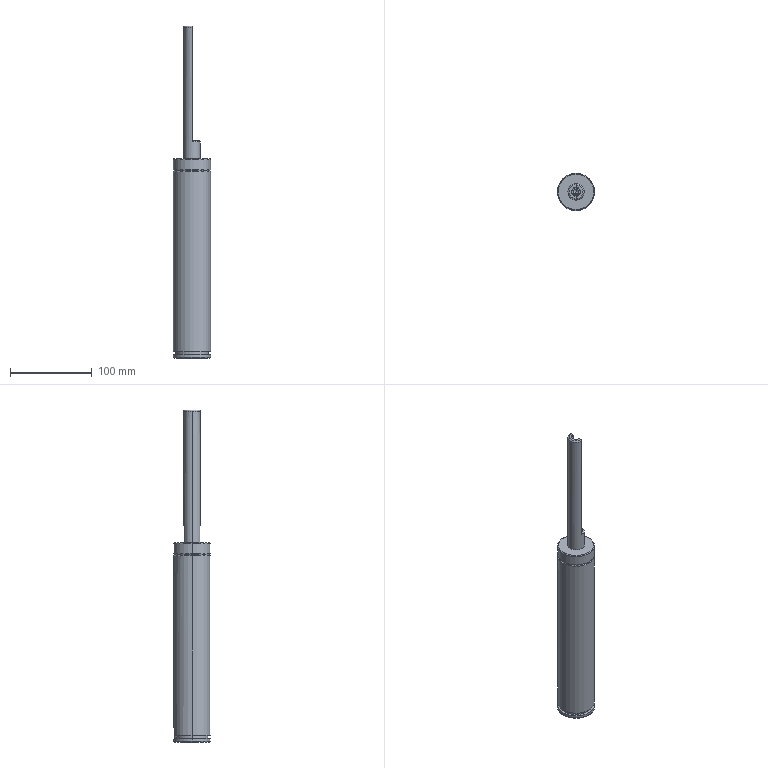Part | STEP file | 1_id3922_x_t | 1 solid | 225 faces | box 45.2 x 45.2 x 405 mm | volume 414792 mm3 | plane 136 | other 48 | cylinder 27 | cone 8 | torus 6 | commonest cylinder face diameters 6.6 x6 14 x6 45.2 x6 39.1 x3 10 x2 16.4 x2